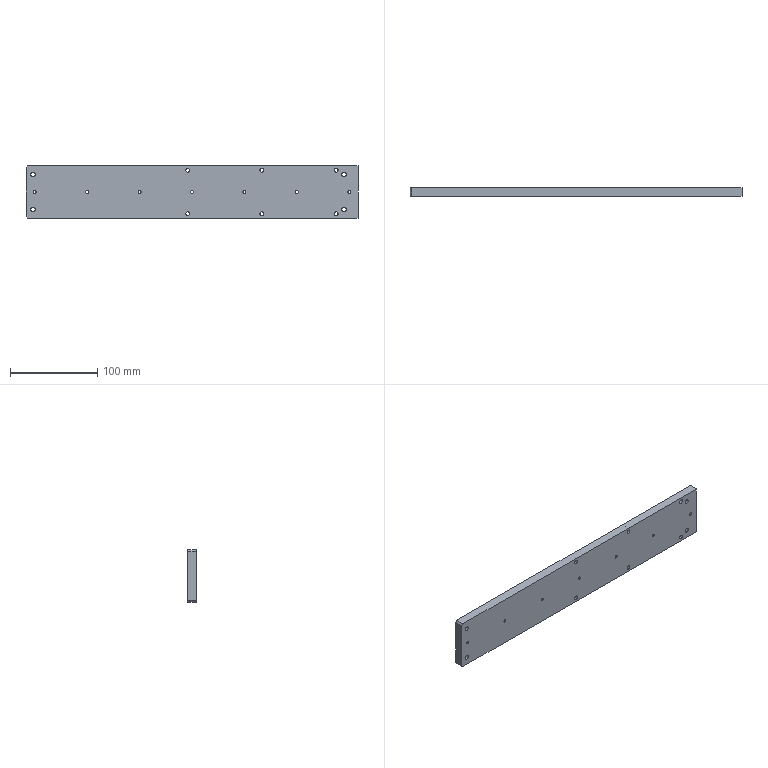Part | SolidWorks | features BaseBody 1 | 1 solid | 68 faces | box 380 x 10 x 60 mm | volume 224318 mm3 | cylinder 50 | plane 14 | cone 4 | commonest cylinder face diameters 3.3 x14 4.5 x12 8 x12 5 x8 4.2 x4